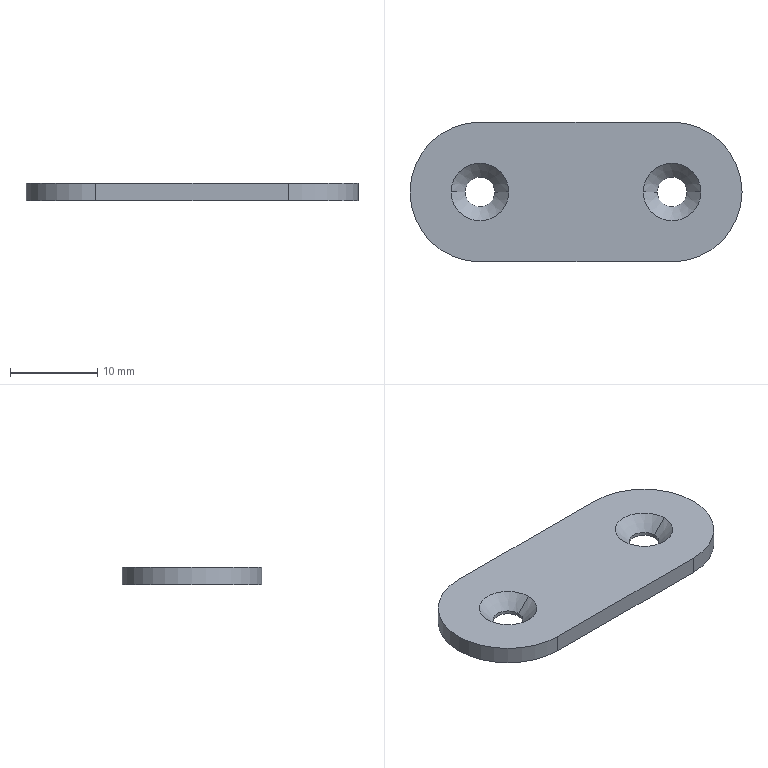Part | SolidWorks | features FlatPattern 1, HoleWzd 1, SMBaseFlange 1, SheetMetal 1 | 1 solid | 15 faces | box 38 x 16 x 2 mm | volume 1034 mm3 | cylinder 7 | cone 4 | plane 4 | commonest cylinder face diameters 3.4 x4 16 x3
STEP:
#1=CARTESIAN_POINT('',(-10.97,0.,-1.6));
#2=VERTEX_POINT('',#1);
#3=CARTESIAN_POINT('',(-7.57,0.,-1.6));
#4=VERTEX_POINT('',#3);
#5=CARTESIAN_POINT('',(-9.27,0.,-1.6));
#6=DIRECTION('',(0.,0.,1.));
#7=DIRECTION('',(1.,0.,0.));
#8=AXIS2_PLACEMENT_3D('',#5,#6,#7);
#9=CIRCLE('',#8,1.7);
#10=EDGE_CURVE('',#2,#4,#9,.T.);
#11=ORIENTED_EDGE('',*,*,#10,.F.);
#12=CARTESIAN_POINT('',(-12.57,0.,0.));
#13=VERTEX_POINT('',#12);
#14=CARTESIAN_POINT('',(-12.57,0.,0.));
#15=DIRECTION('',(-0.7071,0.,0.7071));
#16=VECTOR('',#15,1000.);
#17=LINE('',#14,#16);
#18=EDGE_CURVE('',#2,#13,#17,.T.);
#19=ORIENTED_EDGE('',*,*,#18,.T.);
#20=CARTESIAN_POINT('',(-5.97,0.,0.));
#21=VERTEX_POINT('',#20);
#22=CARTESIAN_POINT('',(-9.27,0.,0.));
#23=DIRECTION('',(0.,0.,1.));
#24=DIRECTION('',(1.,0.,0.));
#25=AXIS2_PLACEMENT_3D('',#22,#23,#24);
#26=CIRCLE('',#25,3.3);
#27=EDGE_CURVE('',#13,#21,#26,.T.);
#28=ORIENTED_EDGE('',*,*,#27,.T.);
#29=CARTESIAN_POINT('',(-5.97,0.,0.));
#30=DIRECTION('',(0.7071,0.,0.7071));
#31=VECTOR('',#30,1000.);
#32=LINE('',#29,#31);
#33=EDGE_CURVE('',#4,#21,#32,.T.);
#34=ORIENTED_EDGE('',*,*,#33,.F.);
#35=EDGE_LOOP('',(#11,#19,#28,#34));
#36=FACE_OUTER_BOUND('',#35,.T.);
#37=CARTESIAN_POINT('',(-9.27,0.,0.));
#38=DIRECTION('',(0.,0.,1.));
#39=DIRECTION('',(1.,0.,0.));
#40=AXIS2_PLACEMENT_3D('',#37,#38,#39);
#41=CONICAL_SURFACE('',#40,3.3,0.7854);
#42=ADVANCED_FACE('',(#36),#41,.F.);
#43=CARTESIAN_POINT('',(-10.97,0.,-2.));
#44=VERTEX_POINT('',#43);
#45=CARTESIAN_POINT('',(-7.57,0.,-2.));
#46=VERTEX_POINT('',#45);
#47=CARTESIAN_POINT('',(-9.27,0.,-2.));
#48=DIRECTION('',(0.,0.,1.));
#49=DIRECTION('',(1.,0.,0.));
#50=AXIS2_PLACEMENT_3D('',#47,#48,#49);
#51=CIRCLE('',#50,1.7);
#52=EDGE_CURVE('',#44,#46,#51,.T.);
#53=ORIENTED_EDGE('',*,*,#52,.F.);
#54=CARTESIAN_POINT('',(-10.97,0.,0.));
#55=DIRECTION('',(0.,0.,1.));
#56=VECTOR('',#55,1000.);
#57=LINE('',#54,#56);
#58=EDGE_CURVE('',#44,#2,#57,.T.);
#59=ORIENTED_EDGE('',*,*,#58,.T.);
#60=ORIENTED_EDGE('',*,*,#10,.T.);
#61=CARTESIAN_POINT('',(-7.57,0.,0.));
#62=DIRECTION('',(0.,0.,1.));
#63=VECTOR('',#62,1000.);
#64=LINE('',#61,#63);
#65=EDGE_CURVE('',#46,#4,#64,.T.);
#66=ORIENTED_EDGE('',*,*,#65,.F.);
#67=EDGE_LOOP('',(#53,#59,#60,#66));
#68=FACE_OUTER_BOUND('',#67,.T.);
#69=CARTESIAN_POINT('',(-9.27,0.,0.));
#70=DIRECTION('',(0.,0.,1.));
#71=DIRECTION('',(1.,0.,0.));
#72=AXIS2_PLACEMENT_3D('',#69,#70,#71);
#73=CYLINDRICAL_SURFACE('',#72,1.7);
#74=ADVANCED_FACE('',(#68),#73,.F.);
#75=CARTESIAN_POINT('',(11.03,0.,-1.6));
#76=VERTEX_POINT('',#75);
#77=CARTESIAN_POINT('',(14.43,0.,-1.6));
#78=VERTEX_POINT('',#77);
#79=CARTESIAN_POINT('',(12.73,0.,-1.6));
#80=DIRECTION('',(0.,0.,1.));
#81=DIRECTION('',(1.,0.,0.));
#82=AXIS2_PLACEMENT_3D('',#79,#80,#81);
#83=CIRCLE('',#82,1.7);
#84=EDGE_CURVE('',#76,#78,#83,.T.);
#85=ORIENTED_EDGE('',*,*,#84,.F.);
#86=CARTESIAN_POINT('',(9.43,0.,0.));
#87=VERTEX_POINT('',#86);
#88=CARTESIAN_POINT('',(9.43,0.,0.));
#89=DIRECTION('',(-0.7071,0.,0.7071));
#90=VECTOR('',#89,1000.);
#91=LINE('',#88,#90);
#92=EDGE_CURVE('',#76,#87,#91,.T.);
#93=ORIENTED_EDGE('',*,*,#92,.T.);
#94=CARTESIAN_POINT('',(16.03,0.,0.));
#95=VERTEX_POINT('',#94);
#96=CARTESIAN_POINT('',(12.73,0.,0.));
#97=DIRECTION('',(0.,0.,1.));
#98=DIRECTION('',(1.,0.,0.));
#99=AXIS2_PLACEMENT_3D('',#96,#97,#98);
#100=CIRCLE('',#99,3.3);
#101=EDGE_CURVE('',#87,#95,#100,.T.);
#102=ORIENTED_EDGE('',*,*,#101,.T.);
#103=CARTESIAN_POINT('',(16.03,0.,0.));
#104=DIRECTION('',(0.7071,0.,0.7071));
#105=VECTOR('',#104,1000.);
#106=LINE('',#103,#105);
#107=EDGE_CURVE('',#78,#95,#106,.T.);
#108=ORIENTED_EDGE('',*,*,#107,.F.);
#109=EDGE_LOOP('',(#85,#93,#102,#108));
#110=FACE_OUTER_BOUND('',#109,.T.);
#111=CARTESIAN_POINT('',(12.73,0.,0.));
#112=DIRECTION('',(0.,0.,1.));
#113=DIRECTION('',(1.,0.,0.));
#114=AXIS2_PLACEMENT_3D('',#111,#112,#113);
#115=CONICAL_SURFACE('',#114,3.3,0.7854);
#116=ADVANCED_FACE('',(#110),#115,.F.);
#117=CARTESIAN_POINT('',(11.03,0.,-2.));
#118=VERTEX_POINT('',#117);
#119=CARTESIAN_POINT('',(14.43,0.,-2.));
#120=VERTEX_POINT('',#119);
#121=CARTESIAN_POINT('',(12.73,0.,-2.));
#122=DIRECTION('',(0.,0.,1.));
#123=DIRECTION('',(1.,0.,0.));
#124=AXIS2_PLACEMENT_3D('',#121,#122,#123);
#125=CIRCLE('',#124,1.7);
#126=EDGE_CURVE('',#118,#120,#125,.T.);
#127=ORIENTED_EDGE('',*,*,#126,.F.);
#128=CARTESIAN_POINT('',(11.03,0.,0.));
#129=DIRECTION('',(0.,0.,1.));
#130=VECTOR('',#129,1000.);
#131=LINE('',#128,#130);
#132=EDGE_CURVE('',#118,#76,#131,.T.);
#133=ORIENTED_EDGE('',*,*,#132,.T.);
#134=ORIENTED_EDGE('',*,*,#84,.T.);
#135=CARTESIAN_POINT('',(14.43,0.,0.));
#136=DIRECTION('',(0.,0.,1.));
#137=VECTOR('',#136,1000.);
#138=LINE('',#135,#137);
#139=EDGE_CURVE('',#120,#78,#138,.T.);
#140=ORIENTED_EDGE('',*,*,#139,.F.);
#141=EDGE_LOOP('',(#127,#133,#134,#140));
#142=FACE_OUTER_BOUND('',#141,.T.);
#143=CARTESIAN_POINT('',(12.73,0.,0.));
#144=DIRECTION('',(0.,0.,1.));
#145=DIRECTION('',(1.,0.,0.));
#146=AXIS2_PLACEMENT_3D('',#143,#144,#145);
#147=CYLINDRICAL_SURFACE('',#146,1.7);
#148=ADVANCED_FACE('',(#142),#147,.F.);
#149=CARTESIAN_POINT('',(12.73,-8.,-2.));
#150=VERTEX_POINT('',#149);
#151=CARTESIAN_POINT('',(20.73,0.,-2.));
#152=VERTEX_POINT('',#151);
#153=CARTESIAN_POINT('',(12.73,0.,-2.));
#154=DIRECTION('',(0.,0.,1.));
#155=DIRECTION('',(1.,0.,0.));
#156=AXIS2_PLACEMENT_3D('',#153,#154,#155);
#157=CIRCLE('',#156,8.);
#158=EDGE_CURVE('',#150,#152,#157,.T.);
#159=ORIENTED_EDGE('',*,*,#158,.T.);
#160=CARTESIAN_POINT('',(20.73,0.,0.));
#161=VERTEX_POINT('',#160);
#162=CARTESIAN_POINT('',(20.73,0.,-2.));
#163=DIRECTION('',(0.,0.,1.));
#164=VECTOR('',#163,1000.);
#165=LINE('',#162,#164);
#166=EDGE_CURVE('',#152,#161,#165,.T.);
#167=ORIENTED_EDGE('',*,*,#166,.T.);
#168=CARTESIAN_POINT('',(12.73,-8.,0.));
#169=VERTEX_POINT('',#168);
#170=CARTESIAN_POINT('',(12.73,0.,0.));
#171=DIRECTION('',(0.,0.,1.));
#172=DIRECTION('',(1.,0.,0.));
#173=AXIS2_PLACEMENT_3D('',#170,#171,#172);
#174=CIRCLE('',#173,8.);
#175=EDGE_CURVE('',#169,#161,#174,.T.);
#176=ORIENTED_EDGE('',*,*,#175,.F.);
#177=CARTESIAN_POINT('',(12.73,-8.,-2.));
#178=DIRECTION('',(0.,0.,1.));
#179=VECTOR('',#178,1000.);
#180=LINE('',#177,#179);
#181=EDGE_CURVE('',#150,#169,#180,.T.);
#182=ORIENTED_EDGE('',*,*,#181,.F.);
#183=EDGE_LOOP('',(#159,#167,#176,#182));
#184=FACE_OUTER_BOUND('',#183,.T.);
#185=CARTESIAN_POINT('',(12.73,0.,-2.));
#186=DIRECTION('',(0.,0.,1.));
#187=DIRECTION('',(1.,0.,0.));
#188=AXIS2_PLACEMENT_3D('',#185,#186,#187);
#189=CYLINDRICAL_SURFACE('',#188,8.);
#190=ADVANCED_FACE('',(#184),#189,.T.);
#191=CARTESIAN_POINT('',(-9.27,8.,0.));
#192=VERTEX_POINT('',#191);
#193=CARTESIAN_POINT('',(-9.27,-8.,0.));
#194=VERTEX_POINT('',#193);
#195=CARTESIAN_POINT('',(-9.27,0.,0.));
#196=DIRECTION('',(0.,0.,1.));
#197=DIRECTION('',(1.,0.,0.));
#198=AXIS2_PLACEMENT_3D('',#195,#196,#197);
#199=CIRCLE('',#198,8.);
#200=EDGE_CURVE('',#192,#194,#199,.T.);
#201=ORIENTED_EDGE('',*,*,#200,.F.);
#202=CARTESIAN_POINT('',(-9.27,8.,-2.));
#203=VERTEX_POINT('',#202);
#204=CARTESIAN_POINT('',(-9.27,8.,-2.));
#205=DIRECTION('',(0.,0.,1.));
#206=VECTOR('',#205,1000.);
#207=LINE('',#204,#206);
#208=EDGE_CURVE('',#203,#192,#207,.T.);
#209=ORIENTED_EDGE('',*,*,#208,.F.);
#210=CARTESIAN_POINT('',(-9.27,-8.,-2.));
#211=VERTEX_POINT('',#210);
#212=CARTESIAN_POINT('',(-9.27,0.,-2.));
#213=DIRECTION('',(0.,0.,1.));
#214=DIRECTION('',(1.,0.,0.));
#215=AXIS2_PLACEMENT_3D('',#212,#213,#214);
#216=CIRCLE('',#215,8.);
#217=EDGE_CURVE('',#203,#211,#216,.T.);
#218=ORIENTED_EDGE('',*,*,#217,.T.);
#219=CARTESIAN_POINT('',(-9.27,-8.,-2.));
#220=DIRECTION('',(0.,0.,1.));
#221=VECTOR('',#220,1000.);
#222=LINE('',#219,#221);
#223=EDGE_CURVE('',#211,#194,#222,.T.);
#224=ORIENTED_EDGE('',*,*,#223,.T.);
#225=EDGE_LOOP('',(#201,#209,#218,#224));
#226=FACE_OUTER_BOUND('',#225,.T.);
#227=CARTESIAN_POINT('',(-9.27,0.,-2.));
#228=DIRECTION('',(0.,0.,1.));
#229=DIRECTION('',(1.,0.,0.));
#230=AXIS2_PLACEMENT_3D('',#227,#228,#229);
#231=CYLINDRICAL_SURFACE('',#230,8.);
#232=ADVANCED_FACE('',(#226),#231,.T.);
#233=CARTESIAN_POINT('',(12.73,8.,0.));
#234=VERTEX_POINT('',#233);
#235=CARTESIAN_POINT('',(-9.27,8.,0.));
#236=DIRECTION('',(-1.,0.,0.));
#237=VECTOR('',#236,1000.);
#238=LINE('',#235,#237);
#239=EDGE_CURVE('',#234,#192,#238,.T.);
#240=ORIENTED_EDGE('',*,*,#239,.F.);
#241=CARTESIAN_POINT('',(12.73,8.,-2.));
#242=VERTEX_POINT('',#241);
#243=CARTESIAN_POINT('',(12.73,8.,-2.));
#244=DIRECTION('',(0.,0.,1.));
#245=VECTOR('',#244,1000.);
#246=LINE('',#243,#245);
#247=EDGE_CURVE('',#242,#234,#246,.T.);
#248=ORIENTED_EDGE('',*,*,#247,.F.);
#249=CARTESIAN_POINT('',(-9.27,8.,-2.));
#250=DIRECTION('',(-1.,0.,0.));
#251=VECTOR('',#250,1000.);
#252=LINE('',#249,#251);
#253=EDGE_CURVE('',#242,#203,#252,.T.);
#254=ORIENTED_EDGE('',*,*,#253,.T.);
#255=ORIENTED_EDGE('',*,*,#208,.T.);
#256=EDGE_LOOP('',(#240,#248,#254,#255));
#257=FACE_OUTER_BOUND('',#256,.T.);
#258=CARTESIAN_POINT('',(-9.27,8.,-2.));
#259=DIRECTION('',(0.,1.,0.));
#260=DIRECTION('',(0.,0.,1.));
#261=AXIS2_PLACEMENT_3D('',#258,#259,#260);
#262=PLANE('',#261);
#263=ADVANCED_FACE('',(#257),#262,.T.);
#264=ORIENTED_EDGE('',*,*,#166,.F.);
#265=CARTESIAN_POINT('',(12.73,0.,-2.));
#266=DIRECTION('',(0.,0.,1.));
#267=DIRECTION('',(1.,0.,0.));
#268=AXIS2_PLACEMENT_3D('',#265,#266,#267);
#269=CIRCLE('',#268,8.);
#270=EDGE_CURVE('',#152,#242,#269,.T.);
#271=ORIENTED_EDGE('',*,*,#270,.T.);
#272=ORIENTED_EDGE('',*,*,#247,.T.);
#273=CARTESIAN_POINT('',(12.73,0.,0.));
#274=DIRECTION('',(0.,0.,1.));
#275=DIRECTION('',(1.,0.,0.));
#276=AXIS2_PLACEMENT_3D('',#273,#274,#275);
#277=CIRCLE('',#276,8.);
#278=EDGE_CURVE('',#161,#234,#277,.T.);
#279=ORIENTED_EDGE('',*,*,#278,.F.);
#280=EDGE_LOOP('',(#264,#271,#272,#279));
#281=FACE_OUTER_BOUND('',#280,.T.);
#282=CARTESIAN_POINT('',(12.73,0.,-2.));
#283=DIRECTION('',(0.,0.,1.));
#284=DIRECTION('',(1.,0.,0.));
#285=AXIS2_PLACEMENT_3D('',#282,#283,#284);
#286=CYLINDRICAL_SURFACE('',#285,8.);
#287=ADVANCED_FACE('',(#281),#286,.T.);
#288=CARTESIAN_POINT('',(-9.27,-8.,0.));
#289=DIRECTION('',(1.,0.,0.));
#290=VECTOR('',#289,1000.);
#291=LINE('',#288,#290);
#292=EDGE_CURVE('',#194,#169,#291,.T.);
#293=ORIENTED_EDGE('',*,*,#292,.F.);
#294=ORIENTED_EDGE('',*,*,#223,.F.);
#295=CARTESIAN_POINT('',(-9.27,-8.,-2.));
#296=DIRECTION('',(1.,0.,0.));
#297=VECTOR('',#296,1000.);
#298=LINE('',#295,#297);
#299=EDGE_CURVE('',#211,#150,#298,.T.);
#300=ORIENTED_EDGE('',*,*,#299,.T.);
#301=ORIENTED_EDGE('',*,*,#181,.T.);
#302=EDGE_LOOP('',(#293,#294,#300,#301));
#303=FACE_OUTER_BOUND('',#302,.T.);
#304=CARTESIAN_POINT('',(-9.27,-8.,-2.));
#305=DIRECTION('',(0.,-1.,0.));
#306=DIRECTION('',(0.,0.,-1.));
#307=AXIS2_PLACEMENT_3D('',#304,#305,#306);
#308=PLANE('',#307);
#309=ADVANCED_FACE('',(#303),#308,.T.);
#310=CARTESIAN_POINT('',(-9.27,0.,-2.));
#311=DIRECTION('',(0.,0.,1.));
#312=DIRECTION('',(1.,0.,0.));
#313=AXIS2_PLACEMENT_3D('',#310,#311,#312);
#314=CIRCLE('',#313,1.7);
#315=EDGE_CURVE('',#46,#44,#314,.T.);
#316=ORIENTED_EDGE('',*,*,#315,.T.);
#317=ORIENTED_EDGE('',*,*,#52,.T.);
#318=EDGE_LOOP('',(#316,#317));
#319=FACE_BOUND('',#318,.T.);
#320=CARTESIAN_POINT('',(12.73,0.,-2.));
#321=DIRECTION('',(0.,0.,1.));
#322=DIRECTION('',(1.,0.,0.));
#323=AXIS2_PLACEMENT_3D('',#320,#321,#322);
#324=CIRCLE('',#323,1.7);
#325=EDGE_CURVE('',#120,#118,#324,.T.);
#326=ORIENTED_EDGE('',*,*,#325,.T.);
#327=ORIENTED_EDGE('',*,*,#126,.T.);
#328=EDGE_LOOP('',(#326,#327));
#329=FACE_BOUND('',#328,.T.);
#330=ORIENTED_EDGE('',*,*,#217,.F.);
#331=ORIENTED_EDGE('',*,*,#253,.F.);
#332=ORIENTED_EDGE('',*,*,#270,.F.);
#333=ORIENTED_EDGE('',*,*,#158,.F.);
#334=ORIENTED_EDGE('',*,*,#299,.F.);
#335=EDGE_LOOP('',(#330,#331,#332,#333,#334));
#336=FACE_OUTER_BOUND('',#335,.T.);
#337=CARTESIAN_POINT('',(-9.27,0.,-2.));
#338=DIRECTION('',(0.,0.,1.));
#339=DIRECTION('',(1.,0.,0.));
#340=AXIS2_PLACEMENT_3D('',#337,#338,#339);
#341=PLANE('',#340);
#342=ADVANCED_FACE('',(#319,#329,#336),#341,.F.);
#343=CARTESIAN_POINT('',(-9.27,0.,0.));
#344=DIRECTION('',(0.,0.,1.));
#345=DIRECTION('',(1.,0.,0.));
#346=AXIS2_PLACEMENT_3D('',#343,#344,#345);
#347=CIRCLE('',#346,3.3);
#348=EDGE_CURVE('',#21,#13,#347,.T.);
#349=ORIENTED_EDGE('',*,*,#348,.F.);
#350=ORIENTED_EDGE('',*,*,#27,.F.);
#351=EDGE_LOOP('',(#349,#350));
#352=FACE_BOUND('',#351,.T.);
#353=CARTESIAN_POINT('',(12.73,0.,0.));
#354=DIRECTION('',(0.,0.,1.));
#355=DIRECTION('',(1.,0.,0.));
#356=AXIS2_PLACEMENT_3D('',#353,#354,#355);
#357=CIRCLE('',#356,3.3);
#358=EDGE_CURVE('',#95,#87,#357,.T.);
#359=ORIENTED_EDGE('',*,*,#358,.F.);
#360=ORIENTED_EDGE('',*,*,#101,.F.);
#361=EDGE_LOOP('',(#359,#360));
#362=FACE_BOUND('',#361,.T.);
#363=ORIENTED_EDGE('',*,*,#200,.T.);
#364=ORIENTED_EDGE('',*,*,#292,.T.);
#365=ORIENTED_EDGE('',*,*,#175,.T.);
#366=ORIENTED_EDGE('',*,*,#278,.T.);
#367=ORIENTED_EDGE('',*,*,#239,.T.);
#368=EDGE_LOOP('',(#363,#364,#365,#366,#367));
#369=FACE_OUTER_BOUND('',#368,.T.);
#370=CARTESIAN_POINT('',(-9.27,0.,0.));
#371=DIRECTION('',(0.,0.,1.));
#372=DIRECTION('',(1.,0.,0.));
#373=AXIS2_PLACEMENT_3D('',#370,#371,#372);
#374=PLANE('',#373);
#375=ADVANCED_FACE('',(#352,#362,#369),#374,.T.);
#376=ORIENTED_EDGE('',*,*,#132,.F.);
#377=ORIENTED_EDGE('',*,*,#325,.F.);
#378=ORIENTED_EDGE('',*,*,#139,.T.);
#379=CARTESIAN_POINT('',(12.73,0.,-1.6));
#380=DIRECTION('',(0.,0.,1.));
#381=DIRECTION('',(1.,0.,0.));
#382=AXIS2_PLACEMENT_3D('',#379,#380,#381);
#383=CIRCLE('',#382,1.7);
#384=EDGE_CURVE('',#78,#76,#383,.T.);
#385=ORIENTED_EDGE('',*,*,#384,.T.);
#386=EDGE_LOOP('',(#376,#377,#378,#385));
#387=FACE_OUTER_BOUND('',#386,.T.);
#388=CARTESIAN_POINT('',(12.73,0.,0.));
#389=DIRECTION('',(0.,0.,1.));
#390=DIRECTION('',(1.,0.,0.));
#391=AXIS2_PLACEMENT_3D('',#388,#389,#390);
#392=CYLINDRICAL_SURFACE('',#391,1.7);
#393=ADVANCED_FACE('',(#387),#392,.F.);
#394=ORIENTED_EDGE('',*,*,#92,.F.);
#395=ORIENTED_EDGE('',*,*,#384,.F.);
#396=ORIENTED_EDGE('',*,*,#107,.T.);
#397=ORIENTED_EDGE('',*,*,#358,.T.);
#398=EDGE_LOOP('',(#394,#395,#396,#397));
#399=FACE_OUTER_BOUND('',#398,.T.);
#400=CARTESIAN_POINT('',(12.73,0.,0.));
#401=DIRECTION('',(0.,0.,1.));
#402=DIRECTION('',(1.,0.,0.));
#403=AXIS2_PLACEMENT_3D('',#400,#401,#402);
#404=CONICAL_SURFACE('',#403,3.3,0.7854);
#405=ADVANCED_FACE('',(#399),#404,.F.);
#406=ORIENTED_EDGE('',*,*,#58,.F.);
#407=ORIENTED_EDGE('',*,*,#315,.F.);
#408=ORIENTED_EDGE('',*,*,#65,.T.);
#409=CARTESIAN_POINT('',(-9.27,0.,-1.6));
#410=DIRECTION('',(0.,0.,1.));
#411=DIRECTION('',(1.,0.,0.));
#412=AXIS2_PLACEMENT_3D('',#409,#410,#411);
#413=CIRCLE('',#412,1.7);
#414=EDGE_CURVE('',#4,#2,#413,.T.);
#415=ORIENTED_EDGE('',*,*,#414,.T.);
#416=EDGE_LOOP('',(#406,#407,#408,#415));
#417=FACE_OUTER_BOUND('',#416,.T.);
#418=CARTESIAN_POINT('',(-9.27,0.,0.));
#419=DIRECTION('',(0.,0.,1.));
#420=DIRECTION('',(1.,0.,0.));
#421=AXIS2_PLACEMENT_3D('',#418,#419,#420);
#422=CYLINDRICAL_SURFACE('',#421,1.7);
#423=ADVANCED_FACE('',(#417),#422,.F.);
#424=ORIENTED_EDGE('',*,*,#18,.F.);
#425=ORIENTED_EDGE('',*,*,#414,.F.);
#426=ORIENTED_EDGE('',*,*,#33,.T.);
#427=ORIENTED_EDGE('',*,*,#348,.T.);
#428=EDGE_LOOP('',(#424,#425,#426,#427));
#429=FACE_OUTER_BOUND('',#428,.T.);
#430=CARTESIAN_POINT('',(-9.27,0.,0.));
#431=DIRECTION('',(0.,0.,1.));
#432=DIRECTION('',(1.,0.,0.));
#433=AXIS2_PLACEMENT_3D('',#430,#431,#432);
#434=CONICAL_SURFACE('',#433,3.3,0.7854);
#435=ADVANCED_FACE('',(#429),#434,.F.);
#436=CLOSED_SHELL('',(#42,#74,#116,#148,#190,#232,#263,#287,#309,#342,#375,#393,#405,#423,#435));
#437=MANIFOLD_SOLID_BREP('',#436);
#438=CARTESIAN_POINT('',(0.,0.,0.));
#439=DIRECTION('',(0.,0.,1.));
#440=DIRECTION('',(1.,0.,0.));
#441=AXIS2_PLACEMENT_3D('',#438,#439,#440);
#442=(LENGTH_UNIT()NAMED_UNIT(*)SI_UNIT(.MILLI.,.METRE.));
#443=UNCERTAINTY_MEASURE_WITH_UNIT(LENGTH_MEASURE(0.00001),#442,'','');
#444=(NAMED_UNIT(*)PLANE_ANGLE_UNIT()SI_UNIT($,.RADIAN.));
#445=(NAMED_UNIT(*)SI_UNIT($,.STERADIAN.)SOLID_ANGLE_UNIT());
#446=(GEOMETRIC_REPRESENTATION_CONTEXT(3)GLOBAL_UNCERTAINTY_ASSIGNED_CONTEXT((#443))GLOBAL_UNIT_ASSIGNED_CONTEXT((#442,#444,#445))REPRESENTATION_CONTEXT('',''));
#447=ADVANCED_BREP_SHAPE_REPRESENTATION('',(#437,#441),#446);